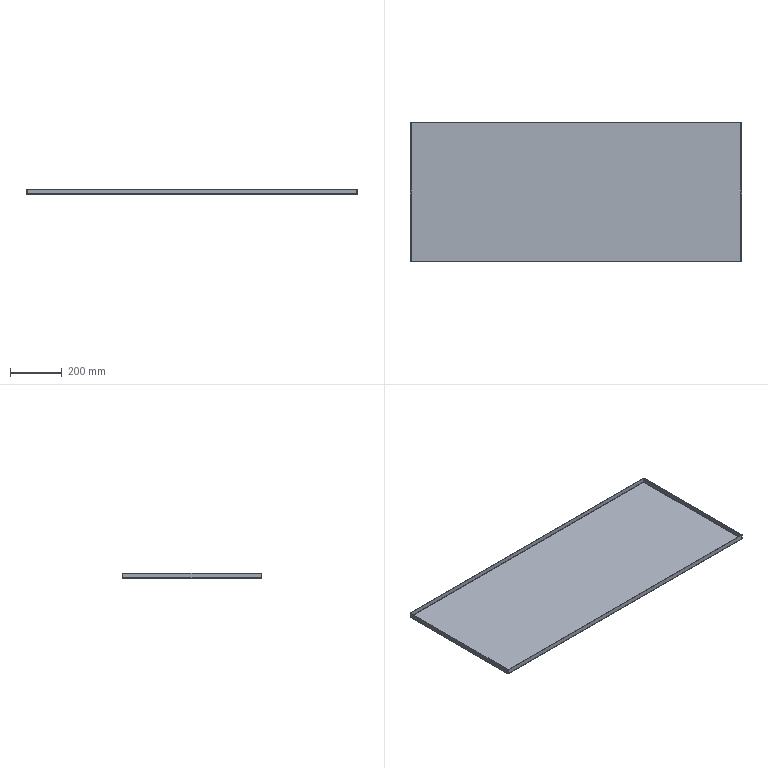Part | STEP file | Part 9 | 1 solid | 38 faces | box 1280 x 540 x 20 mm | volume 1507947 mm3 | plane 22 | spline 8 | cylinder 8 | commonest cylinder face diameters 1 x4 5 x4
STEP:
#1=CARTESIAN_POINT('',(-637.5,-267.5,-2.));
#2=VERTEX_POINT('',#1);
#3=CARTESIAN_POINT('',(-637.5,267.5,-2.));
#4=VERTEX_POINT('',#3);
#5=CARTESIAN_POINT('',(-637.5,-267.5,-2.));
#6=DIRECTION('',(0.,1.,0.));
#7=VECTOR('',#6,1000.);
#8=LINE('',#5,#7);
#9=EDGE_CURVE('',#2,#4,#8,.T.);
#10=ORIENTED_EDGE('',*,*,#9,.T.);
#11=CARTESIAN_POINT('',(637.5,267.5,-2.));
#12=VERTEX_POINT('',#11);
#13=CARTESIAN_POINT('',(-637.5,267.5,-2.));
#14=DIRECTION('',(1.,0.,0.));
#15=VECTOR('',#14,1000.);
#16=LINE('',#13,#15);
#17=EDGE_CURVE('',#4,#12,#16,.T.);
#18=ORIENTED_EDGE('',*,*,#17,.T.);
#19=CARTESIAN_POINT('',(637.5,-267.5,-2.));
#20=VERTEX_POINT('',#19);
#21=CARTESIAN_POINT('',(637.5,267.5,-2.));
#22=DIRECTION('',(0.,-1.,0.));
#23=VECTOR('',#22,1000.);
#24=LINE('',#21,#23);
#25=EDGE_CURVE('',#12,#20,#24,.T.);
#26=ORIENTED_EDGE('',*,*,#25,.T.);
#27=CARTESIAN_POINT('',(637.5,-267.5,-2.));
#28=DIRECTION('',(-1.,0.,0.));
#29=VECTOR('',#28,1000.);
#30=LINE('',#27,#29);
#31=EDGE_CURVE('',#20,#2,#30,.T.);
#32=ORIENTED_EDGE('',*,*,#31,.T.);
#33=EDGE_LOOP('',(#10,#18,#26,#32));
#34=FACE_OUTER_BOUND('',#33,.T.);
#35=CARTESIAN_POINT('',(0.,0.,-2.));
#36=DIRECTION('',(0.,0.,1.));
#37=DIRECTION('',(1.,0.,0.));
#38=AXIS2_PLACEMENT_3D('',#35,#36,#37);
#39=PLANE('',#38);
#40=ADVANCED_FACE('',(#34),#39,.F.);
#41=CARTESIAN_POINT('',(-637.5,267.5,0.));
#42=VERTEX_POINT('',#41);
#43=CARTESIAN_POINT('',(637.5,267.5,0.));
#44=VERTEX_POINT('',#43);
#45=CARTESIAN_POINT('',(-637.5,267.5,0.));
#46=DIRECTION('',(1.,0.,0.));
#47=VECTOR('',#46,1000.);
#48=LINE('',#45,#47);
#49=EDGE_CURVE('',#42,#44,#48,.T.);
#50=ORIENTED_EDGE('',*,*,#49,.F.);
#51=CARTESIAN_POINT('',(-637.5,-267.5,0.));
#52=VERTEX_POINT('',#51);
#53=CARTESIAN_POINT('',(-637.5,-267.5,0.));
#54=DIRECTION('',(0.,1.,0.));
#55=VECTOR('',#54,1000.);
#56=LINE('',#53,#55);
#57=EDGE_CURVE('',#52,#42,#56,.T.);
#58=ORIENTED_EDGE('',*,*,#57,.F.);
#59=CARTESIAN_POINT('',(637.5,-267.5,0.));
#60=VERTEX_POINT('',#59);
#61=CARTESIAN_POINT('',(637.5,-267.5,0.));
#62=DIRECTION('',(-1.,0.,0.));
#63=VECTOR('',#62,1000.);
#64=LINE('',#61,#63);
#65=EDGE_CURVE('',#60,#52,#64,.T.);
#66=ORIENTED_EDGE('',*,*,#65,.F.);
#67=CARTESIAN_POINT('',(637.5,267.5,0.));
#68=DIRECTION('',(0.,-1.,0.));
#69=VECTOR('',#68,1000.);
#70=LINE('',#67,#69);
#71=EDGE_CURVE('',#44,#60,#70,.T.);
#72=ORIENTED_EDGE('',*,*,#71,.F.);
#73=EDGE_LOOP('',(#50,#58,#66,#72));
#74=FACE_OUTER_BOUND('',#73,.T.);
#75=CARTESIAN_POINT('',(0.,0.,0.));
#76=DIRECTION('',(0.,0.,1.));
#77=DIRECTION('',(1.,0.,0.));
#78=AXIS2_PLACEMENT_3D('',#75,#76,#77);
#79=PLANE('',#78);
#80=ADVANCED_FACE('',(#74),#79,.T.);
#81=CARTESIAN_POINT('',(637.293,270.,0.5));
#82=VERTEX_POINT('',#81);
#83=CARTESIAN_POINT('',(637.293,268.,0.5));
#84=VERTEX_POINT('',#83);
#85=CARTESIAN_POINT('',(637.293,268.,0.5));
#86=DIRECTION('',(0.,-1.,0.));
#87=VECTOR('',#86,1000.);
#88=LINE('',#85,#87);
#89=EDGE_CURVE('',#82,#84,#88,.T.);
#90=ORIENTED_EDGE('',*,*,#89,.T.);
#91=CARTESIAN_POINT('',(637.5,267.5,0.));
#92=CARTESIAN_POINT('',(637.465,267.631,0.));
#93=CARTESIAN_POINT('',(637.431,267.761,0.05389));
#94=CARTESIAN_POINT('',(637.362,267.946,0.239));
#95=CARTESIAN_POINT('',(637.327,268.,0.3691));
#96=CARTESIAN_POINT('',(637.293,268.,0.5));
#97=B_SPLINE_CURVE_WITH_KNOTS('',3,(#91,#92,#93,#94,#95,#96),.UNSPECIFIED.,.F.,.F.,(4,2,4),(0.,0.5,1.),.UNSPECIFIED.);
#98=EDGE_CURVE('',#44,#84,#97,.T.);
#99=ORIENTED_EDGE('',*,*,#98,.F.);
#100=CARTESIAN_POINT('',(637.5,267.5,0.));
#101=DIRECTION('',(0.,0.,-1.));
#102=VECTOR('',#101,1000.);
#103=LINE('',#100,#102);
#104=EDGE_CURVE('',#44,#12,#103,.T.);
#105=ORIENTED_EDGE('',*,*,#104,.T.);
#106=CARTESIAN_POINT('',(637.5,267.5,-2.));
#107=CARTESIAN_POINT('',(637.483,267.827,-2.));
#108=CARTESIAN_POINT('',(637.465,268.154,-1.935));
#109=CARTESIAN_POINT('',(637.431,268.759,-1.684));
#110=CARTESIAN_POINT('',(637.414,269.036,-1.499));
#111=CARTESIAN_POINT('',(637.379,269.499,-1.036));
#112=CARTESIAN_POINT('',(637.362,269.684,-0.759));
#113=CARTESIAN_POINT('',(637.327,269.935,-0.1544));
#114=CARTESIAN_POINT('',(637.31,270.,0.1728));
#115=CARTESIAN_POINT('',(637.293,270.,0.5));
#116=B_SPLINE_CURVE_WITH_KNOTS('',3,(#106,#107,#108,#109,#110,#111,#112,#113,#114,#115),.UNSPECIFIED.,.F.,.F.,(4,2,2,2,4),(0.,0.25,0.5,0.75,1.),.UNSPECIFIED.);
#117=EDGE_CURVE('',#12,#82,#116,.T.);
#118=ORIENTED_EDGE('',*,*,#117,.T.);
#119=EDGE_LOOP('',(#90,#99,#105,#118));
#120=FACE_OUTER_BOUND('',#119,.T.);
#121=CARTESIAN_POINT('',(637.5,267.5,-2.02));
#122=CARTESIAN_POINT('',(637.483,267.83,-2.02));
#123=CARTESIAN_POINT('',(637.465,268.16,-1.954));
#124=CARTESIAN_POINT('',(637.431,268.769,-1.702));
#125=CARTESIAN_POINT('',(637.414,269.049,-1.515));
#126=CARTESIAN_POINT('',(637.379,269.515,-1.049));
#127=CARTESIAN_POINT('',(637.362,269.702,-0.7691));
#128=CARTESIAN_POINT('',(637.327,269.954,-0.1596));
#129=CARTESIAN_POINT('',(637.31,270.02,0.1701));
#130=CARTESIAN_POINT('',(637.293,270.02,0.5));
#131=CARTESIAN_POINT('',(637.5,267.5,-2.));
#132=CARTESIAN_POINT('',(637.483,267.827,-2.));
#133=CARTESIAN_POINT('',(637.465,268.154,-1.935));
#134=CARTESIAN_POINT('',(637.431,268.759,-1.684));
#135=CARTESIAN_POINT('',(637.414,269.036,-1.499));
#136=CARTESIAN_POINT('',(637.379,269.499,-1.036));
#137=CARTESIAN_POINT('',(637.362,269.684,-0.759));
#138=CARTESIAN_POINT('',(637.327,269.935,-0.1544));
#139=CARTESIAN_POINT('',(637.31,270.,0.1727));
#140=CARTESIAN_POINT('',(637.293,270.,0.5));
#141=CARTESIAN_POINT('',(637.5,267.5,0.));
#142=CARTESIAN_POINT('',(637.483,267.565,0.));
#143=CARTESIAN_POINT('',(637.465,267.631,0.01301));
#144=CARTESIAN_POINT('',(637.431,267.752,0.06311));
#145=CARTESIAN_POINT('',(637.414,267.807,0.1002));
#146=CARTESIAN_POINT('',(637.379,267.9,0.1927));
#147=CARTESIAN_POINT('',(637.362,267.937,0.2482));
#148=CARTESIAN_POINT('',(637.327,267.987,0.3691));
#149=CARTESIAN_POINT('',(637.31,268.,0.4345));
#150=CARTESIAN_POINT('',(637.293,268.,0.5));
#151=CARTESIAN_POINT('',(637.5,267.5,0.0202));
#152=CARTESIAN_POINT('',(637.483,267.563,0.0202));
#153=CARTESIAN_POINT('',(637.465,267.626,0.03269));
#154=CARTESIAN_POINT('',(637.431,267.742,0.08076));
#155=CARTESIAN_POINT('',(637.414,267.795,0.1163));
#156=CARTESIAN_POINT('',(637.379,267.884,0.2051));
#157=CARTESIAN_POINT('',(637.362,267.919,0.2584));
#158=CARTESIAN_POINT('',(637.327,267.967,0.3744));
#159=CARTESIAN_POINT('',(637.31,267.98,0.4372));
#160=CARTESIAN_POINT('',(637.293,267.98,0.5));
#161=B_SPLINE_SURFACE_WITH_KNOTS('',1,3,((#121,#122,#123,#124,#125,#126,#127,#128,#129,#130),(#131,#132,#133,#134,#135,#136,#137,#138,#139,#140),(#141,#142,#143,#144,#145,#146,#147,#148,#149,#150),(#151,#152,#153,#154,#155,#156,#157,#158,#159,#160)),.UNSPECIFIED.,.F.,.F.,.F.,(2,1,1,2),(4,2,2,2,4),(-0.01,0.,1.,1.01),(0.,0.25,0.5,0.75,1.),.UNSPECIFIED.);
#162=ADVANCED_FACE('',(#120),#161,.F.);
#163=CARTESIAN_POINT('',(-637.293,268.,0.5));
#164=VERTEX_POINT('',#163);
#165=CARTESIAN_POINT('',(-637.293,268.,0.5));
#166=CARTESIAN_POINT('',(-637.327,268.,0.3691));
#167=CARTESIAN_POINT('',(-637.362,267.946,0.239));
#168=CARTESIAN_POINT('',(-637.431,267.761,0.05389));
#169=CARTESIAN_POINT('',(-637.465,267.631,0.));
#170=CARTESIAN_POINT('',(-637.5,267.5,0.));
#171=B_SPLINE_CURVE_WITH_KNOTS('',3,(#165,#166,#167,#168,#169,#170),.UNSPECIFIED.,.F.,.F.,(4,2,4),(0.,0.5,1.),.UNSPECIFIED.);
#172=EDGE_CURVE('',#164,#42,#171,.T.);
#173=ORIENTED_EDGE('',*,*,#172,.F.);
#174=CARTESIAN_POINT('',(-637.293,270.,0.5));
#175=VERTEX_POINT('',#174);
#176=CARTESIAN_POINT('',(-637.293,268.,0.5));
#177=DIRECTION('',(0.,-1.,0.));
#178=VECTOR('',#177,1000.);
#179=LINE('',#176,#178);
#180=EDGE_CURVE('',#175,#164,#179,.T.);
#181=ORIENTED_EDGE('',*,*,#180,.F.);
#182=CARTESIAN_POINT('',(-637.293,270.,0.5));
#183=CARTESIAN_POINT('',(-637.31,270.,0.1728));
#184=CARTESIAN_POINT('',(-637.327,269.935,-0.1544));
#185=CARTESIAN_POINT('',(-637.362,269.684,-0.759));
#186=CARTESIAN_POINT('',(-637.379,269.499,-1.036));
#187=CARTESIAN_POINT('',(-637.414,269.036,-1.499));
#188=CARTESIAN_POINT('',(-637.431,268.759,-1.684));
#189=CARTESIAN_POINT('',(-637.465,268.154,-1.935));
#190=CARTESIAN_POINT('',(-637.483,267.827,-2.));
#191=CARTESIAN_POINT('',(-637.5,267.5,-2.));
#192=B_SPLINE_CURVE_WITH_KNOTS('',3,(#182,#183,#184,#185,#186,#187,#188,#189,#190,#191),.UNSPECIFIED.,.F.,.F.,(4,2,2,2,4),(0.,0.25,0.5,0.75,1.),.UNSPECIFIED.);
#193=EDGE_CURVE('',#175,#4,#192,.T.);
#194=ORIENTED_EDGE('',*,*,#193,.T.);
#195=CARTESIAN_POINT('',(-637.5,267.5,0.));
#196=DIRECTION('',(0.,0.,-1.));
#197=VECTOR('',#196,1000.);
#198=LINE('',#195,#197);
#199=EDGE_CURVE('',#42,#4,#198,.T.);
#200=ORIENTED_EDGE('',*,*,#199,.F.);
#201=EDGE_LOOP('',(#173,#181,#194,#200));
#202=FACE_OUTER_BOUND('',#201,.T.);
#203=CARTESIAN_POINT('',(-637.293,270.02,0.5));
#204=CARTESIAN_POINT('',(-637.31,270.02,0.1701));
#205=CARTESIAN_POINT('',(-637.327,269.954,-0.1596));
#206=CARTESIAN_POINT('',(-637.362,269.702,-0.7691));
#207=CARTESIAN_POINT('',(-637.379,269.515,-1.049));
#208=CARTESIAN_POINT('',(-637.414,269.049,-1.515));
#209=CARTESIAN_POINT('',(-637.431,268.769,-1.702));
#210=CARTESIAN_POINT('',(-637.465,268.16,-1.954));
#211=CARTESIAN_POINT('',(-637.483,267.83,-2.02));
#212=CARTESIAN_POINT('',(-637.5,267.5,-2.02));
#213=CARTESIAN_POINT('',(-637.293,270.,0.5));
#214=CARTESIAN_POINT('',(-637.31,270.,0.1727));
#215=CARTESIAN_POINT('',(-637.327,269.935,-0.1544));
#216=CARTESIAN_POINT('',(-637.362,269.684,-0.759));
#217=CARTESIAN_POINT('',(-637.379,269.499,-1.036));
#218=CARTESIAN_POINT('',(-637.414,269.036,-1.499));
#219=CARTESIAN_POINT('',(-637.431,268.759,-1.684));
#220=CARTESIAN_POINT('',(-637.465,268.154,-1.935));
#221=CARTESIAN_POINT('',(-637.483,267.827,-2.));
#222=CARTESIAN_POINT('',(-637.5,267.5,-2.));
#223=CARTESIAN_POINT('',(-637.293,268.,0.5));
#224=CARTESIAN_POINT('',(-637.31,268.,0.4345));
#225=CARTESIAN_POINT('',(-637.327,267.987,0.3691));
#226=CARTESIAN_POINT('',(-637.362,267.937,0.2482));
#227=CARTESIAN_POINT('',(-637.379,267.9,0.1927));
#228=CARTESIAN_POINT('',(-637.414,267.807,0.1002));
#229=CARTESIAN_POINT('',(-637.431,267.752,0.06311));
#230=CARTESIAN_POINT('',(-637.465,267.631,0.01301));
#231=CARTESIAN_POINT('',(-637.483,267.565,0.));
#232=CARTESIAN_POINT('',(-637.5,267.5,0.));
#233=CARTESIAN_POINT('',(-637.293,267.98,0.5));
#234=CARTESIAN_POINT('',(-637.31,267.98,0.4372));
#235=CARTESIAN_POINT('',(-637.327,267.967,0.3744));
#236=CARTESIAN_POINT('',(-637.362,267.919,0.2584));
#237=CARTESIAN_POINT('',(-637.379,267.884,0.2051));
#238=CARTESIAN_POINT('',(-637.414,267.795,0.1163));
#239=CARTESIAN_POINT('',(-637.431,267.742,0.08076));
#240=CARTESIAN_POINT('',(-637.465,267.626,0.03269));
#241=CARTESIAN_POINT('',(-637.483,267.563,0.0202));
#242=CARTESIAN_POINT('',(-637.5,267.5,0.0202));
#243=B_SPLINE_SURFACE_WITH_KNOTS('',1,3,((#203,#204,#205,#206,#207,#208,#209,#210,#211,#212),(#213,#214,#215,#216,#217,#218,#219,#220,#221,#222),(#223,#224,#225,#226,#227,#228,#229,#230,#231,#232),(#233,#234,#235,#236,#237,#238,#239,#240,#241,#242)),.UNSPECIFIED.,.F.,.F.,.F.,(2,1,1,2),(4,2,2,2,4),(-0.01,0.,1.,1.01),(0.,0.25,0.5,0.75,1.),.UNSPECIFIED.);
#244=ADVANCED_FACE('',(#202),#243,.F.);
#245=ORIENTED_EDGE('',*,*,#17,.F.);
#246=ORIENTED_EDGE('',*,*,#193,.F.);
#247=CARTESIAN_POINT('',(0.,270.,0.5));
#248=DIRECTION('',(-1.,0.,0.));
#249=VECTOR('',#248,1000.);
#250=LINE('',#247,#249);
#251=EDGE_CURVE('',#82,#175,#250,.T.);
#252=ORIENTED_EDGE('',*,*,#251,.F.);
#253=ORIENTED_EDGE('',*,*,#117,.F.);
#254=EDGE_LOOP('',(#245,#246,#252,#253));
#255=FACE_OUTER_BOUND('',#254,.T.);
#256=CARTESIAN_POINT('',(-637.5,267.5,0.5));
#257=DIRECTION('',(-1.,0.,0.));
#258=DIRECTION('',(0.,1.,0.));
#259=AXIS2_PLACEMENT_3D('',#256,#257,#258);
#260=CYLINDRICAL_SURFACE('',#259,2.5);
#261=ADVANCED_FACE('',(#255),#260,.T.);
#262=ORIENTED_EDGE('',*,*,#49,.T.);
#263=ORIENTED_EDGE('',*,*,#98,.T.);
#264=CARTESIAN_POINT('',(640.,268.,0.5));
#265=DIRECTION('',(-1.,0.,0.));
#266=VECTOR('',#265,1000.);
#267=LINE('',#264,#266);
#268=EDGE_CURVE('',#84,#164,#267,.T.);
#269=ORIENTED_EDGE('',*,*,#268,.T.);
#270=ORIENTED_EDGE('',*,*,#172,.T.);
#271=EDGE_LOOP('',(#262,#263,#269,#270));
#272=FACE_OUTER_BOUND('',#271,.T.);
#273=CARTESIAN_POINT('',(-637.5,267.5,0.5));
#274=DIRECTION('',(-1.,0.,0.));
#275=DIRECTION('',(0.,1.,0.));
#276=AXIS2_PLACEMENT_3D('',#273,#274,#275);
#277=CYLINDRICAL_SURFACE('',#276,0.5);
#278=ADVANCED_FACE('',(#272),#277,.F.);
#279=CARTESIAN_POINT('',(637.293,268.,18.));
#280=VERTEX_POINT('',#279);
#281=CARTESIAN_POINT('',(637.293,270.,18.));
#282=VERTEX_POINT('',#281);
#283=CARTESIAN_POINT('',(637.293,270.,18.));
#284=DIRECTION('',(0.,1.,0.));
#285=VECTOR('',#284,1000.);
#286=LINE('',#283,#285);
#287=EDGE_CURVE('',#280,#282,#286,.T.);
#288=ORIENTED_EDGE('',*,*,#287,.F.);
#289=CARTESIAN_POINT('',(637.293,268.,0.));
#290=DIRECTION('',(0.,0.,1.));
#291=VECTOR('',#290,1000.);
#292=LINE('',#289,#291);
#293=EDGE_CURVE('',#84,#280,#292,.T.);
#294=ORIENTED_EDGE('',*,*,#293,.F.);
#295=ORIENTED_EDGE('',*,*,#89,.F.);
#296=CARTESIAN_POINT('',(637.293,270.,0.));
#297=DIRECTION('',(0.,0.,-1.));
#298=VECTOR('',#297,1000.);
#299=LINE('',#296,#298);
#300=EDGE_CURVE('',#282,#82,#299,.T.);
#301=ORIENTED_EDGE('',*,*,#300,.F.);
#302=EDGE_LOOP('',(#288,#294,#295,#301));
#303=FACE_OUTER_BOUND('',#302,.T.);
#304=CARTESIAN_POINT('',(637.293,268.,0.));
#305=DIRECTION('',(1.,0.,0.));
#306=DIRECTION('',(0.,0.,-1.));
#307=AXIS2_PLACEMENT_3D('',#304,#305,#306);
#308=PLANE('',#307);
#309=ADVANCED_FACE('',(#303),#308,.T.);
#310=CARTESIAN_POINT('',(-637.293,270.,18.));
#311=VERTEX_POINT('',#310);
#312=CARTESIAN_POINT('',(-637.293,270.,0.));
#313=DIRECTION('',(0.,0.,-1.));
#314=VECTOR('',#313,1000.);
#315=LINE('',#312,#314);
#316=EDGE_CURVE('',#311,#175,#315,.T.);
#317=ORIENTED_EDGE('',*,*,#316,.F.);
#318=CARTESIAN_POINT('',(-640.,270.,18.));
#319=DIRECTION('',(-1.,0.,0.));
#320=VECTOR('',#319,1000.);
#321=LINE('',#318,#320);
#322=EDGE_CURVE('',#282,#311,#321,.T.);
#323=ORIENTED_EDGE('',*,*,#322,.F.);
#324=ORIENTED_EDGE('',*,*,#300,.T.);
#325=ORIENTED_EDGE('',*,*,#251,.T.);
#326=EDGE_LOOP('',(#317,#323,#324,#325));
#327=FACE_OUTER_BOUND('',#326,.T.);
#328=CARTESIAN_POINT('',(0.,270.,0.));
#329=DIRECTION('',(0.,1.,0.));
#330=DIRECTION('',(0.,0.,1.));
#331=AXIS2_PLACEMENT_3D('',#328,#329,#330);
#332=PLANE('',#331);
#333=ADVANCED_FACE('',(#327),#332,.T.);
#334=CARTESIAN_POINT('',(-637.293,268.,18.));
#335=VERTEX_POINT('',#334);
#336=CARTESIAN_POINT('',(0.,268.,18.));
#337=DIRECTION('',(-1.,0.,0.));
#338=VECTOR('',#337,1000.);
#339=LINE('',#336,#338);
#340=EDGE_CURVE('',#280,#335,#339,.T.);
#341=ORIENTED_EDGE('',*,*,#340,.T.);
#342=CARTESIAN_POINT('',(-637.293,268.,0.));
#343=DIRECTION('',(0.,0.,1.));
#344=VECTOR('',#343,1000.);
#345=LINE('',#342,#344);
#346=EDGE_CURVE('',#164,#335,#345,.T.);
#347=ORIENTED_EDGE('',*,*,#346,.F.);
#348=ORIENTED_EDGE('',*,*,#268,.F.);
#349=ORIENTED_EDGE('',*,*,#293,.T.);
#350=EDGE_LOOP('',(#341,#347,#348,#349));
#351=FACE_OUTER_BOUND('',#350,.T.);
#352=CARTESIAN_POINT('',(0.,268.,0.));
#353=DIRECTION('',(0.,1.,0.));
#354=DIRECTION('',(0.,0.,1.));
#355=AXIS2_PLACEMENT_3D('',#352,#353,#354);
#356=PLANE('',#355);
#357=ADVANCED_FACE('',(#351),#356,.F.);
#358=CARTESIAN_POINT('',(-637.293,268.,18.));
#359=DIRECTION('',(0.,1.,0.));
#360=VECTOR('',#359,1000.);
#361=LINE('',#358,#360);
#362=EDGE_CURVE('',#335,#311,#361,.T.);
#363=ORIENTED_EDGE('',*,*,#362,.F.);
#364=ORIENTED_EDGE('',*,*,#340,.F.);
#365=ORIENTED_EDGE('',*,*,#287,.T.);
#366=ORIENTED_EDGE('',*,*,#322,.T.);
#367=EDGE_LOOP('',(#363,#364,#365,#366));
#368=FACE_OUTER_BOUND('',#367,.T.);
#369=CARTESIAN_POINT('',(-640.,270.,18.));
#370=DIRECTION('',(0.,0.,1.));
#371=DIRECTION('',(0.,-1.,0.));
#372=AXIS2_PLACEMENT_3D('',#369,#370,#371);
#373=PLANE('',#372);
#374=ADVANCED_FACE('',(#368),#373,.T.);
#375=ORIENTED_EDGE('',*,*,#346,.T.);
#376=ORIENTED_EDGE('',*,*,#362,.T.);
#377=ORIENTED_EDGE('',*,*,#316,.T.);
#378=ORIENTED_EDGE('',*,*,#180,.T.);
#379=EDGE_LOOP('',(#375,#376,#377,#378));
#380=FACE_OUTER_BOUND('',#379,.T.);
#381=CARTESIAN_POINT('',(-637.293,268.,0.));
#382=DIRECTION('',(1.,0.,0.));
#383=DIRECTION('',(0.,0.,-1.));
#384=AXIS2_PLACEMENT_3D('',#381,#382,#383);
#385=PLANE('',#384);
#386=ADVANCED_FACE('',(#380),#385,.F.);
#387=CARTESIAN_POINT('',(640.,-267.293,0.5));
#388=VERTEX_POINT('',#387);
#389=CARTESIAN_POINT('',(638.,-267.293,0.5));
#390=VERTEX_POINT('',#389);
#391=CARTESIAN_POINT('',(638.,-267.293,0.5));
#392=DIRECTION('',(-1.,0.,0.));
#393=VECTOR('',#392,1000.);
#394=LINE('',#391,#393);
#395=EDGE_CURVE('',#388,#390,#394,.T.);
#396=ORIENTED_EDGE('',*,*,#395,.T.);
#397=CARTESIAN_POINT('',(637.5,-267.5,0.));
#398=CARTESIAN_POINT('',(637.631,-267.465,0.));
#399=CARTESIAN_POINT('',(637.761,-267.431,0.05389));
#400=CARTESIAN_POINT('',(637.946,-267.362,0.239));
#401=CARTESIAN_POINT('',(638.,-267.327,0.3691));
#402=CARTESIAN_POINT('',(638.,-267.293,0.5));
#403=B_SPLINE_CURVE_WITH_KNOTS('',3,(#397,#398,#399,#400,#401,#402),.UNSPECIFIED.,.F.,.F.,(4,2,4),(0.,0.5,1.),.UNSPECIFIED.);
#404=EDGE_CURVE('',#60,#390,#403,.T.);
#405=ORIENTED_EDGE('',*,*,#404,.F.);
#406=CARTESIAN_POINT('',(637.5,-267.5,0.));
#407=DIRECTION('',(0.,0.,-1.));
#408=VECTOR('',#407,1000.);
#409=LINE('',#406,#408);
#410=EDGE_CURVE('',#60,#20,#409,.T.);
#411=ORIENTED_EDGE('',*,*,#410,.T.);
#412=CARTESIAN_POINT('',(637.5,-267.5,-2.));
#413=CARTESIAN_POINT('',(637.827,-267.483,-2.));
#414=CARTESIAN_POINT('',(638.154,-267.465,-1.935));
#415=CARTESIAN_POINT('',(638.759,-267.431,-1.684));
#416=CARTESIAN_POINT('',(639.036,-267.414,-1.499));
#417=CARTESIAN_POINT('',(639.499,-267.379,-1.036));
#418=CARTESIAN_POINT('',(639.684,-267.362,-0.759));
#419=CARTESIAN_POINT('',(639.935,-267.327,-0.1544));
#420=CARTESIAN_POINT('',(640.,-267.31,0.1728));
#421=CARTESIAN_POINT('',(640.,-267.293,0.5));
#422=B_SPLINE_CURVE_WITH_KNOTS('',3,(#412,#413,#414,#415,#416,#417,#418,#419,#420,#421),.UNSPECIFIED.,.F.,.F.,(4,2,2,2,4),(0.,0.25,0.5,0.75,1.),.UNSPECIFIED.);
#423=EDGE_CURVE('',#20,#388,#422,.T.);
#424=ORIENTED_EDGE('',*,*,#423,.T.);
#425=EDGE_LOOP('',(#396,#405,#411,#424));
#426=FACE_OUTER_BOUND('',#425,.T.);
#427=CARTESIAN_POINT('',(637.5,-267.5,-2.02));
#428=CARTESIAN_POINT('',(637.83,-267.483,-2.02));
#429=CARTESIAN_POINT('',(638.16,-267.465,-1.954));
#430=CARTESIAN_POINT('',(638.769,-267.431,-1.702));
#431=CARTESIAN_POINT('',(639.049,-267.414,-1.515));
#432=CARTESIAN_POINT('',(639.515,-267.379,-1.049));
#433=CARTESIAN_POINT('',(639.702,-267.362,-0.7691));
#434=CARTESIAN_POINT('',(639.954,-267.327,-0.1596));
#435=CARTESIAN_POINT('',(640.02,-267.31,0.1701));
#436=CARTESIAN_POINT('',(640.02,-267.293,0.5));
#437=CARTESIAN_POINT('',(637.5,-267.5,-2.));
#438=CARTESIAN_POINT('',(637.827,-267.483,-2.));
#439=CARTESIAN_POINT('',(638.154,-267.465,-1.935));
#440=CARTESIAN_POINT('',(638.759,-267.431,-1.684));
#441=CARTESIAN_POINT('',(639.036,-267.414,-1.499));
#442=CARTESIAN_POINT('',(639.499,-267.379,-1.036));
#443=CARTESIAN_POINT('',(639.684,-267.362,-0.759));
#444=CARTESIAN_POINT('',(639.935,-267.327,-0.1544));
#445=CARTESIAN_POINT('',(640.,-267.31,0.1727));
#446=CARTESIAN_POINT('',(640.,-267.293,0.5));
#447=CARTESIAN_POINT('',(637.5,-267.5,0.));
#448=CARTESIAN_POINT('',(637.565,-267.483,0.));
#449=CARTESIAN_POINT('',(637.631,-267.465,0.01301));
#450=CARTESIAN_POINT('',(637.752,-267.431,0.06311));
#451=CARTESIAN_POINT('',(637.807,-267.414,0.1002));
#452=CARTESIAN_POINT('',(637.9,-267.379,0.1927));
#453=CARTESIAN_POINT('',(637.937,-267.362,0.2482));
#454=CARTESIAN_POINT('',(637.987,-267.327,0.3691));
#455=CARTESIAN_POINT('',(638.,-267.31,0.4345));
#456=CARTESIAN_POINT('',(638.,-267.293,0.5));
#457=CARTESIAN_POINT('',(637.5,-267.5,0.0202));
#458=CARTESIAN_POINT('',(637.563,-267.483,0.0202));
#459=CARTESIAN_POINT('',(637.626,-267.465,0.03269));
#460=CARTESIAN_POINT('',(637.742,-267.431,0.08076));
#461=CARTESIAN_POINT('',(637.795,-267.414,0.1163));
#462=CARTESIAN_POINT('',(637.884,-267.379,0.2051));
#463=CARTESIAN_POINT('',(637.919,-267.362,0.2584));
#464=CARTESIAN_POINT('',(637.967,-267.327,0.3744));
#465=CARTESIAN_POINT('',(637.98,-267.31,0.4372));
#466=CARTESIAN_POINT('',(637.98,-267.293,0.5));
#467=B_SPLINE_SURFACE_WITH_KNOTS('',1,3,((#427,#428,#429,#430,#431,#432,#433,#434,#435,#436),(#437,#438,#439,#440,#441,#442,#443,#444,#445,#446),(#447,#448,#449,#450,#451,#452,#453,#454,#455,#456),(#457,#458,#459,#460,#461,#462,#463,#464,#465,#466)),.UNSPECIFIED.,.F.,.F.,.F.,(2,1,1,2),(4,2,2,2,4),(-0.01,0.,1.,1.01),(0.,0.25,0.5,0.75,1.),.UNSPECIFIED.);
#468=ADVANCED_FACE('',(#426),#467,.F.);
#469=CARTESIAN_POINT('',(638.,267.293,0.5));
#470=VERTEX_POINT('',#469);
#471=CARTESIAN_POINT('',(638.,267.293,0.5));
#472=CARTESIAN_POINT('',(638.,267.327,0.3691));
#473=CARTESIAN_POINT('',(637.946,267.362,0.239));
#474=CARTESIAN_POINT('',(637.761,267.431,0.05389));
#475=CARTESIAN_POINT('',(637.631,267.465,0.));
#476=CARTESIAN_POINT('',(637.5,267.5,0.));
#477=B_SPLINE_CURVE_WITH_KNOTS('',3,(#471,#472,#473,#474,#475,#476),.UNSPECIFIED.,.F.,.F.,(4,2,4),(0.,0.5,1.),.UNSPECIFIED.);
#478=EDGE_CURVE('',#470,#44,#477,.T.);
#479=ORIENTED_EDGE('',*,*,#478,.F.);
#480=CARTESIAN_POINT('',(640.,267.293,0.5));
#481=VERTEX_POINT('',#480);
#482=CARTESIAN_POINT('',(638.,267.293,0.5));
#483=DIRECTION('',(-1.,0.,0.));
#484=VECTOR('',#483,1000.);
#485=LINE('',#482,#484);
#486=EDGE_CURVE('',#481,#470,#485,.T.);
#487=ORIENTED_EDGE('',*,*,#486,.F.);
#488=CARTESIAN_POINT('',(640.,267.293,0.5));
#489=CARTESIAN_POINT('',(640.,267.31,0.1728));
#490=CARTESIAN_POINT('',(639.935,267.327,-0.1544));
#491=CARTESIAN_POINT('',(639.684,267.362,-0.759));
#492=CARTESIAN_POINT('',(639.499,267.379,-1.036));
#493=CARTESIAN_POINT('',(639.036,267.414,-1.499));
#494=CARTESIAN_POINT('',(638.759,267.431,-1.684));
#495=CARTESIAN_POINT('',(638.154,267.465,-1.935));
#496=CARTESIAN_POINT('',(637.827,267.483,-2.));
#497=CARTESIAN_POINT('',(637.5,267.5,-2.));
#498=B_SPLINE_CURVE_WITH_KNOTS('',3,(#488,#489,#490,#491,#492,#493,#494,#495,#496,#497),.UNSPECIFIED.,.F.,.F.,(4,2,2,2,4),(0.,0.25,0.5,0.75,1.),.UNSPECIFIED.);
#499=EDGE_CURVE('',#481,#12,#498,.T.);
#500=ORIENTED_EDGE('',*,*,#499,.T.);
#501=ORIENTED_EDGE('',*,*,#104,.F.);
#502=EDGE_LOOP('',(#479,#487,#500,#501));
#503=FACE_OUTER_BOUND('',#502,.T.);
#504=CARTESIAN_POINT('',(640.02,267.293,0.5));
#505=CARTESIAN_POINT('',(640.02,267.31,0.1701));
#506=CARTESIAN_POINT('',(639.954,267.327,-0.1596));
#507=CARTESIAN_POINT('',(639.702,267.362,-0.7691));
#508=CARTESIAN_POINT('',(639.515,267.379,-1.049));
#509=CARTESIAN_POINT('',(639.049,267.414,-1.515));
#510=CARTESIAN_POINT('',(638.769,267.431,-1.702));
#511=CARTESIAN_POINT('',(638.16,267.465,-1.954));
#512=CARTESIAN_POINT('',(637.83,267.483,-2.02));
#513=CARTESIAN_POINT('',(637.5,267.5,-2.02));
#514=CARTESIAN_POINT('',(640.,267.293,0.5));
#515=CARTESIAN_POINT('',(640.,267.31,0.1727));
#516=CARTESIAN_POINT('',(639.935,267.327,-0.1544));
#517=CARTESIAN_POINT('',(639.684,267.362,-0.759));
#518=CARTESIAN_POINT('',(639.499,267.379,-1.036));
#519=CARTESIAN_POINT('',(639.036,267.414,-1.499));
#520=CARTESIAN_POINT('',(638.759,267.431,-1.684));
#521=CARTESIAN_POINT('',(638.154,267.465,-1.935));
#522=CARTESIAN_POINT('',(637.827,267.483,-2.));
#523=CARTESIAN_POINT('',(637.5,267.5,-2.));
#524=CARTESIAN_POINT('',(638.,267.293,0.5));
#525=CARTESIAN_POINT('',(638.,267.31,0.4345));
#526=CARTESIAN_POINT('',(637.987,267.327,0.3691));
#527=CARTESIAN_POINT('',(637.937,267.362,0.2482));
#528=CARTESIAN_POINT('',(637.9,267.379,0.1927));
#529=CARTESIAN_POINT('',(637.807,267.414,0.1002));
#530=CARTESIAN_POINT('',(637.752,267.431,0.06311));
#531=CARTESIAN_POINT('',(637.631,267.465,0.01301));
#532=CARTESIAN_POINT('',(637.565,267.483,0.));
#533=CARTESIAN_POINT('',(637.5,267.5,0.));
#534=CARTESIAN_POINT('',(637.98,267.293,0.5));
#535=CARTESIAN_POINT('',(637.98,267.31,0.4372));
#536=CARTESIAN_POINT('',(637.967,267.327,0.3744));
#537=CARTESIAN_POINT('',(637.919,267.362,0.2584));
#538=CARTESIAN_POINT('',(637.884,267.379,0.2051));
#539=CARTESIAN_POINT('',(637.795,267.414,0.1163));
#540=CARTESIAN_POINT('',(637.742,267.431,0.08076));
#541=CARTESIAN_POINT('',(637.626,267.465,0.03269));
#542=CARTESIAN_POINT('',(637.563,267.483,0.0202));
#543=CARTESIAN_POINT('',(637.5,267.5,0.0202));
#544=B_SPLINE_SURFACE_WITH_KNOTS('',1,3,((#504,#505,#506,#507,#508,#509,#510,#511,#512,#513),(#514,#515,#516,#517,#518,#519,#520,#521,#522,#523),(#524,#525,#526,#527,#528,#529,#530,#531,#532,#533),(#534,#535,#536,#537,#538,#539,#540,#541,#542,#543)),.UNSPECIFIED.,.F.,.F.,.F.,(2,1,1,2),(4,2,2,2,4),(-0.01,0.,1.,1.01),(0.,0.25,0.5,0.75,1.),.UNSPECIFIED.);
#545=ADVANCED_FACE('',(#503),#544,.F.);
#546=ORIENTED_EDGE('',*,*,#25,.F.);
#547=ORIENTED_EDGE('',*,*,#499,.F.);
#548=CARTESIAN_POINT('',(640.,-270.,0.5));
#549=DIRECTION('',(0.,-1.,0.));
#550=VECTOR('',#549,1000.);
#551=LINE('',#548,#550);
#552=EDGE_CURVE('',#481,#388,#551,.T.);
#553=ORIENTED_EDGE('',*,*,#552,.T.);
#554=ORIENTED_EDGE('',*,*,#423,.F.);
#555=EDGE_LOOP('',(#546,#547,#553,#554));
#556=FACE_OUTER_BOUND('',#555,.T.);
#557=CARTESIAN_POINT('',(637.5,267.5,0.5));
#558=DIRECTION('',(0.,1.,0.));
#559=DIRECTION('',(1.,0.,0.));
#560=AXIS2_PLACEMENT_3D('',#557,#558,#559);
#561=CYLINDRICAL_SURFACE('',#560,2.5);
#562=ADVANCED_FACE('',(#556),#561,.T.);
#563=ORIENTED_EDGE('',*,*,#71,.T.);
#564=ORIENTED_EDGE('',*,*,#404,.T.);
#565=CARTESIAN_POINT('',(638.,-270.,0.5));
#566=DIRECTION('',(0.,1.,0.));
#567=VECTOR('',#566,1000.);
#568=LINE('',#565,#567);
#569=EDGE_CURVE('',#390,#470,#568,.T.);
#570=ORIENTED_EDGE('',*,*,#569,.T.);
#571=ORIENTED_EDGE('',*,*,#478,.T.);
#572=EDGE_LOOP('',(#563,#564,#570,#571));
#573=FACE_OUTER_BOUND('',#572,.T.);
#574=CARTESIAN_POINT('',(637.5,267.5,0.5));
#575=DIRECTION('',(0.,1.,0.));
#576=DIRECTION('',(1.,0.,0.));
#577=AXIS2_PLACEMENT_3D('',#574,#575,#576);
#578=CYLINDRICAL_SURFACE('',#577,0.5);
#579=ADVANCED_FACE('',(#573),#578,.F.);
#580=CARTESIAN_POINT('',(638.,-267.293,18.));
#581=VERTEX_POINT('',#580);
#582=CARTESIAN_POINT('',(640.,-267.293,18.));
#583=VERTEX_POINT('',#582);
#584=CARTESIAN_POINT('',(640.,-267.293,18.));
#585=DIRECTION('',(1.,0.,0.));
#586=VECTOR('',#585,1000.);
#587=LINE('',#584,#586);
#588=EDGE_CURVE('',#581,#583,#587,.T.);
#589=ORIENTED_EDGE('',*,*,#588,.F.);
#590=CARTESIAN_POINT('',(638.,-267.293,0.));
#591=DIRECTION('',(0.,0.,1.));
#592=VECTOR('',#591,1000.);
#593=LINE('',#590,#592);
#594=EDGE_CURVE('',#390,#581,#593,.T.);
#595=ORIENTED_EDGE('',*,*,#594,.F.);
#596=ORIENTED_EDGE('',*,*,#395,.F.);
#597=CARTESIAN_POINT('',(640.,-267.293,0.));
#598=DIRECTION('',(0.,0.,1.));
#599=VECTOR('',#598,1000.);
#600=LINE('',#597,#599);
#601=EDGE_CURVE('',#388,#583,#600,.T.);
#602=ORIENTED_EDGE('',*,*,#601,.T.);
#603=EDGE_LOOP('',(#589,#595,#596,#602));
#604=FACE_OUTER_BOUND('',#603,.T.);
#605=CARTESIAN_POINT('',(638.,-267.293,0.));
#606=DIRECTION('',(0.,-1.,0.));
#607=DIRECTION('',(0.,0.,-1.));
#608=AXIS2_PLACEMENT_3D('',#605,#606,#607);
#609=PLANE('',#608);
#610=ADVANCED_FACE('',(#604),#609,.T.);
#611=ORIENTED_EDGE('',*,*,#552,.F.);
#612=CARTESIAN_POINT('',(640.,267.293,18.));
#613=VERTEX_POINT('',#612);
#614=CARTESIAN_POINT('',(640.,267.293,0.));
#615=DIRECTION('',(0.,0.,1.));
#616=VECTOR('',#615,1000.);
#617=LINE('',#614,#616);
#618=EDGE_CURVE('',#481,#613,#617,.T.);
#619=ORIENTED_EDGE('',*,*,#618,.T.);
#620=CARTESIAN_POINT('',(640.,-270.,18.));
#621=DIRECTION('',(0.,1.,0.));
#622=VECTOR('',#621,1000.);
#623=LINE('',#620,#622);
#624=EDGE_CURVE('',#583,#613,#623,.T.);
#625=ORIENTED_EDGE('',*,*,#624,.F.);
#626=ORIENTED_EDGE('',*,*,#601,.F.);
#627=EDGE_LOOP('',(#611,#619,#625,#626));
#628=FACE_OUTER_BOUND('',#627,.T.);
#629=CARTESIAN_POINT('',(640.,0.,0.));
#630=DIRECTION('',(-1.,0.,0.));
#631=DIRECTION('',(0.,-1.,0.));
#632=AXIS2_PLACEMENT_3D('',#629,#630,#631);
#633=PLANE('',#632);
#634=ADVANCED_FACE('',(#628),#633,.F.);
#635=CARTESIAN_POINT('',(638.,267.293,18.));
#636=VERTEX_POINT('',#635);
#637=CARTESIAN_POINT('',(638.,267.293,0.));
#638=DIRECTION('',(0.,0.,1.));
#639=VECTOR('',#638,1000.);
#640=LINE('',#637,#639);
#641=EDGE_CURVE('',#470,#636,#640,.T.);
#642=ORIENTED_EDGE('',*,*,#641,.F.);
#643=ORIENTED_EDGE('',*,*,#569,.F.);
#644=ORIENTED_EDGE('',*,*,#594,.T.);
#645=CARTESIAN_POINT('',(638.,0.,18.));
#646=DIRECTION('',(0.,1.,0.));
#647=VECTOR('',#646,1000.);
#648=LINE('',#645,#647);
#649=EDGE_CURVE('',#581,#636,#648,.T.);
#650=ORIENTED_EDGE('',*,*,#649,.T.);
#651=EDGE_LOOP('',(#642,#643,#644,#650));
#652=FACE_OUTER_BOUND('',#651,.T.);
#653=CARTESIAN_POINT('',(638.,0.,0.));
#654=DIRECTION('',(-1.,0.,0.));
#655=DIRECTION('',(0.,-1.,0.));
#656=AXIS2_PLACEMENT_3D('',#653,#654,#655);
#657=PLANE('',#656);
#658=ADVANCED_FACE('',(#652),#657,.T.);
#659=CARTESIAN_POINT('',(638.,267.293,18.));
#660=DIRECTION('',(1.,0.,0.));
#661=VECTOR('',#660,1000.);
#662=LINE('',#659,#661);
#663=EDGE_CURVE('',#636,#613,#662,.T.);
#664=ORIENTED_EDGE('',*,*,#663,.F.);
#665=ORIENTED_EDGE('',*,*,#649,.F.);
#666=ORIENTED_EDGE('',*,*,#588,.T.);
#667=ORIENTED_EDGE('',*,*,#624,.T.);
#668=EDGE_LOOP('',(#664,#665,#666,#667));
#669=FACE_OUTER_BOUND('',#668,.T.);
#670=CARTESIAN_POINT('',(640.,-270.,18.));
#671=DIRECTION('',(0.,0.,1.));
#672=DIRECTION('',(1.,0.,0.));
#673=AXIS2_PLACEMENT_3D('',#670,#671,#672);
#674=PLANE('',#673);
#675=ADVANCED_FACE('',(#669),#674,.T.);
#676=ORIENTED_EDGE('',*,*,#641,.T.);
#677=ORIENTED_EDGE('',*,*,#663,.T.);
#678=ORIENTED_EDGE('',*,*,#618,.F.);
#679=ORIENTED_EDGE('',*,*,#486,.T.);
#680=EDGE_LOOP('',(#676,#677,#678,#679));
#681=FACE_OUTER_BOUND('',#680,.T.);
#682=CARTESIAN_POINT('',(638.,267.293,0.));
#683=DIRECTION('',(0.,-1.,0.));
#684=DIRECTION('',(0.,0.,-1.));
#685=AXIS2_PLACEMENT_3D('',#682,#683,#684);
#686=PLANE('',#685);
#687=ADVANCED_FACE('',(#681),#686,.F.);
#688=CARTESIAN_POINT('',(-637.293,-270.,0.5));
#689=VERTEX_POINT('',#688);
#690=CARTESIAN_POINT('',(-637.293,-268.,0.5));
#691=VERTEX_POINT('',#690);
#692=CARTESIAN_POINT('',(-637.293,-268.,0.5));
#693=DIRECTION('',(0.,1.,0.));
#694=VECTOR('',#693,1000.);
#695=LINE('',#692,#694);
#696=EDGE_CURVE('',#689,#691,#695,.T.);
#697=ORIENTED_EDGE('',*,*,#696,.T.);
#698=CARTESIAN_POINT('',(-637.5,-267.5,0.));
#699=CARTESIAN_POINT('',(-637.465,-267.631,0.));
#700=CARTESIAN_POINT('',(-637.431,-267.761,0.05389));
#701=CARTESIAN_POINT('',(-637.362,-267.946,0.239));
#702=CARTESIAN_POINT('',(-637.327,-268.,0.3691));
#703=CARTESIAN_POINT('',(-637.293,-268.,0.5));
#704=B_SPLINE_CURVE_WITH_KNOTS('',3,(#698,#699,#700,#701,#702,#703),.UNSPECIFIED.,.F.,.F.,(4,2,4),(0.,0.5,1.),.UNSPECIFIED.);
#705=EDGE_CURVE('',#52,#691,#704,.T.);
#706=ORIENTED_EDGE('',*,*,#705,.F.);
#707=CARTESIAN_POINT('',(-637.5,-267.5,0.));
#708=DIRECTION('',(0.,0.,-1.));
#709=VECTOR('',#708,1000.);
#710=LINE('',#707,#709);
#711=EDGE_CURVE('',#52,#2,#710,.T.);
#712=ORIENTED_EDGE('',*,*,#711,.T.);
#713=CARTESIAN_POINT('',(-637.5,-267.5,-2.));
#714=CARTESIAN_POINT('',(-637.483,-267.827,-2.));
#715=CARTESIAN_POINT('',(-637.465,-268.154,-1.935));
#716=CARTESIAN_POINT('',(-637.431,-268.759,-1.684));
#717=CARTESIAN_POINT('',(-637.414,-269.036,-1.499));
#718=CARTESIAN_POINT('',(-637.379,-269.499,-1.036));
#719=CARTESIAN_POINT('',(-637.362,-269.684,-0.759));
#720=CARTESIAN_POINT('',(-637.327,-269.935,-0.1544));
#721=CARTESIAN_POINT('',(-637.31,-270.,0.1728));
#722=CARTESIAN_POINT('',(-637.293,-270.,0.5));
#723=B_SPLINE_CURVE_WITH_KNOTS('',3,(#713,#714,#715,#716,#717,#718,#719,#720,#721,#722),.UNSPECIFIED.,.F.,.F.,(4,2,2,2,4),(0.,0.25,0.5,0.75,1.),.UNSPECIFIED.);
#724=EDGE_CURVE('',#2,#689,#723,.T.);
#725=ORIENTED_EDGE('',*,*,#724,.T.);
#726=EDGE_LOOP('',(#697,#706,#712,#725));
#727=FACE_OUTER_BOUND('',#726,.T.);
#728=CARTESIAN_POINT('',(-637.5,-267.5,-2.02));
#729=CARTESIAN_POINT('',(-637.483,-267.83,-2.02));
#730=CARTESIAN_POINT('',(-637.465,-268.16,-1.954));
#731=CARTESIAN_POINT('',(-637.431,-268.769,-1.702));
#732=CARTESIAN_POINT('',(-637.414,-269.049,-1.515));
#733=CARTESIAN_POINT('',(-637.379,-269.515,-1.049));
#734=CARTESIAN_POINT('',(-637.362,-269.702,-0.7691));
#735=CARTESIAN_POINT('',(-637.327,-269.954,-0.1596));
#736=CARTESIAN_POINT('',(-637.31,-270.02,0.1701));
#737=CARTESIAN_POINT('',(-637.293,-270.02,0.5));
#738=CARTESIAN_POINT('',(-637.5,-267.5,-2.));
#739=CARTESIAN_POINT('',(-637.483,-267.827,-2.));
#740=CARTESIAN_POINT('',(-637.465,-268.154,-1.935));
#741=CARTESIAN_POINT('',(-637.431,-268.759,-1.684));
#742=CARTESIAN_POINT('',(-637.414,-269.036,-1.499));
#743=CARTESIAN_POINT('',(-637.379,-269.499,-1.036));
#744=CARTESIAN_POINT('',(-637.362,-269.684,-0.759));
#745=CARTESIAN_POINT('',(-637.327,-269.935,-0.1544));
#746=CARTESIAN_POINT('',(-637.31,-270.,0.1727));
#747=CARTESIAN_POINT('',(-637.293,-270.,0.5));
#748=CARTESIAN_POINT('',(-637.5,-267.5,0.));
#749=CARTESIAN_POINT('',(-637.483,-267.565,0.));
#750=CARTESIAN_POINT('',(-637.465,-267.631,0.01301));
#751=CARTESIAN_POINT('',(-637.431,-267.752,0.06311));
#752=CARTESIAN_POINT('',(-637.414,-267.807,0.1002));
#753=CARTESIAN_POINT('',(-637.379,-267.9,0.1927));
#754=CARTESIAN_POINT('',(-637.362,-267.937,0.2482));
#755=CARTESIAN_POINT('',(-637.327,-267.987,0.3691));
#756=CARTESIAN_POINT('',(-637.31,-268.,0.4345));
#757=CARTESIAN_POINT('',(-637.293,-268.,0.5));
#758=CARTESIAN_POINT('',(-637.5,-267.5,0.0202));
#759=CARTESIAN_POINT('',(-637.483,-267.563,0.0202));
#760=CARTESIAN_POINT('',(-637.465,-267.626,0.03269));
#761=CARTESIAN_POINT('',(-637.431,-267.742,0.08076));
#762=CARTESIAN_POINT('',(-637.414,-267.795,0.1163));
#763=CARTESIAN_POINT('',(-637.379,-267.884,0.2051));
#764=CARTESIAN_POINT('',(-637.362,-267.919,0.2584));
#765=CARTESIAN_POINT('',(-637.327,-267.967,0.3744));
#766=CARTESIAN_POINT('',(-637.31,-267.98,0.4372));
#767=CARTESIAN_POINT('',(-637.293,-267.98,0.5));
#768=B_SPLINE_SURFACE_WITH_KNOTS('',1,3,((#728,#729,#730,#731,#732,#733,#734,#735,#736,#737),(#738,#739,#740,#741,#742,#743,#744,#745,#746,#747),(#748,#749,#750,#751,#752,#753,#754,#755,#756,#757),(#758,#759,#760,#761,#762,#763,#764,#765,#766,#767)),.UNSPECIFIED.,.F.,.F.,.F.,(2,1,1,2),(4,2,2,2,4),(-0.01,0.,1.,1.01),(0.,0.25,0.5,0.75,1.),.UNSPECIFIED.);
#769=ADVANCED_FACE('',(#727),#768,.F.);
#770=CARTESIAN_POINT('',(637.293,-268.,0.5));
#771=VERTEX_POINT('',#770);
#772=CARTESIAN_POINT('',(637.293,-268.,0.5));
#773=CARTESIAN_POINT('',(637.327,-268.,0.3691));
#774=CARTESIAN_POINT('',(637.362,-267.946,0.239));
#775=CARTESIAN_POINT('',(637.431,-267.761,0.05389));
#776=CARTESIAN_POINT('',(637.465,-267.631,0.));
#777=CARTESIAN_POINT('',(637.5,-267.5,0.));
#778=B_SPLINE_CURVE_WITH_KNOTS('',3,(#772,#773,#774,#775,#776,#777),.UNSPECIFIED.,.F.,.F.,(4,2,4),(0.,0.5,1.),.UNSPECIFIED.);
#779=EDGE_CURVE('',#771,#60,#778,.T.);
#780=ORIENTED_EDGE('',*,*,#779,.F.);
#781=CARTESIAN_POINT('',(637.293,-270.,0.5));
#782=VERTEX_POINT('',#781);
#783=CARTESIAN_POINT('',(637.293,-268.,0.5));
#784=DIRECTION('',(0.,1.,0.));
#785=VECTOR('',#784,1000.);
#786=LINE('',#783,#785);
#787=EDGE_CURVE('',#782,#771,#786,.T.);
#788=ORIENTED_EDGE('',*,*,#787,.F.);
#789=CARTESIAN_POINT('',(637.293,-270.,0.5));
#790=CARTESIAN_POINT('',(637.31,-270.,0.1728));
#791=CARTESIAN_POINT('',(637.327,-269.935,-0.1544));
#792=CARTESIAN_POINT('',(637.362,-269.684,-0.759));
#793=CARTESIAN_POINT('',(637.379,-269.499,-1.036));
#794=CARTESIAN_POINT('',(637.414,-269.036,-1.499));
#795=CARTESIAN_POINT('',(637.431,-268.759,-1.684));
#796=CARTESIAN_POINT('',(637.465,-268.154,-1.935));
#797=CARTESIAN_POINT('',(637.483,-267.827,-2.));
#798=CARTESIAN_POINT('',(637.5,-267.5,-2.));
#799=B_SPLINE_CURVE_WITH_KNOTS('',3,(#789,#790,#791,#792,#793,#794,#795,#796,#797,#798),.UNSPECIFIED.,.F.,.F.,(4,2,2,2,4),(0.,0.25,0.5,0.75,1.),.UNSPECIFIED.);
#800=EDGE_CURVE('',#782,#20,#799,.T.);
#801=ORIENTED_EDGE('',*,*,#800,.T.);
#802=ORIENTED_EDGE('',*,*,#410,.F.);
#803=EDGE_LOOP('',(#780,#788,#801,#802));
#804=FACE_OUTER_BOUND('',#803,.T.);
#805=CARTESIAN_POINT('',(637.293,-270.02,0.5));
#806=CARTESIAN_POINT('',(637.31,-270.02,0.1701));
#807=CARTESIAN_POINT('',(637.327,-269.954,-0.1596));
#808=CARTESIAN_POINT('',(637.362,-269.702,-0.7691));
#809=CARTESIAN_POINT('',(637.379,-269.515,-1.049));
#810=CARTESIAN_POINT('',(637.414,-269.049,-1.515));
#811=CARTESIAN_POINT('',(637.431,-268.769,-1.702));
#812=CARTESIAN_POINT('',(637.465,-268.16,-1.954));
#813=CARTESIAN_POINT('',(637.483,-267.83,-2.02));
#814=CARTESIAN_POINT('',(637.5,-267.5,-2.02));
#815=CARTESIAN_POINT('',(637.293,-270.,0.5));
#816=CARTESIAN_POINT('',(637.31,-270.,0.1727));
#817=CARTESIAN_POINT('',(637.327,-269.935,-0.1544));
#818=CARTESIAN_POINT('',(637.362,-269.684,-0.759));
#819=CARTESIAN_POINT('',(637.379,-269.499,-1.036));
#820=CARTESIAN_POINT('',(637.414,-269.036,-1.499));
#821=CARTESIAN_POINT('',(637.431,-268.759,-1.684));
#822=CARTESIAN_POINT('',(637.465,-268.154,-1.935));
#823=CARTESIAN_POINT('',(637.483,-267.827,-2.));
#824=CARTESIAN_POINT('',(637.5,-267.5,-2.));
#825=CARTESIAN_POINT('',(637.293,-268.,0.5));
#826=CARTESIAN_POINT('',(637.31,-268.,0.4345));
#827=CARTESIAN_POINT('',(637.327,-267.987,0.3691));
#828=CARTESIAN_POINT('',(637.362,-267.937,0.2482));
#829=CARTESIAN_POINT('',(637.379,-267.9,0.1927));
#830=CARTESIAN_POINT('',(637.414,-267.807,0.1002));
#831=CARTESIAN_POINT('',(637.431,-267.752,0.06311));
#832=CARTESIAN_POINT('',(637.465,-267.631,0.01301));
#833=CARTESIAN_POINT('',(637.483,-267.565,0.));
#834=CARTESIAN_POINT('',(637.5,-267.5,0.));
#835=CARTESIAN_POINT('',(637.293,-267.98,0.5));
#836=CARTESIAN_POINT('',(637.31,-267.98,0.4372));
#837=CARTESIAN_POINT('',(637.327,-267.967,0.3744));
#838=CARTESIAN_POINT('',(637.362,-267.919,0.2584));
#839=CARTESIAN_POINT('',(637.379,-267.884,0.2051));
#840=CARTESIAN_POINT('',(637.414,-267.795,0.1163));
#841=CARTESIAN_POINT('',(637.431,-267.742,0.08076));
#842=CARTESIAN_POINT('',(637.465,-267.626,0.03269));
#843=CARTESIAN_POINT('',(637.483,-267.563,0.0202));
#844=CARTESIAN_POINT('',(637.5,-267.5,0.0202));
#845=B_SPLINE_SURFACE_WITH_KNOTS('',1,3,((#805,#806,#807,#808,#809,#810,#811,#812,#813,#814),(#815,#816,#817,#818,#819,#820,#821,#822,#823,#824),(#825,#826,#827,#828,#829,#830,#831,#832,#833,#834),(#835,#836,#837,#838,#839,#840,#841,#842,#843,#844)),.UNSPECIFIED.,.F.,.F.,.F.,(2,1,1,2),(4,2,2,2,4),(-0.01,0.,1.,1.01),(0.,0.25,0.5,0.75,1.),.UNSPECIFIED.);
#846=ADVANCED_FACE('',(#804),#845,.F.);
#847=ORIENTED_EDGE('',*,*,#31,.F.);
#848=ORIENTED_EDGE('',*,*,#800,.F.);
#849=CARTESIAN_POINT('',(-640.,-270.,0.5));
#850=DIRECTION('',(-1.,0.,0.));
#851=VECTOR('',#850,1000.);
#852=LINE('',#849,#851);
#853=EDGE_CURVE('',#782,#689,#852,.T.);
#854=ORIENTED_EDGE('',*,*,#853,.T.);
#855=ORIENTED_EDGE('',*,*,#724,.F.);
#856=EDGE_LOOP('',(#847,#848,#854,#855));
#857=FACE_OUTER_BOUND('',#856,.T.);
#858=CARTESIAN_POINT('',(637.5,-267.5,0.5));
#859=DIRECTION('',(1.,0.,0.));
#860=DIRECTION('',(0.,-1.,0.));
#861=AXIS2_PLACEMENT_3D('',#858,#859,#860);
#862=CYLINDRICAL_SURFACE('',#861,2.5);
#863=ADVANCED_FACE('',(#857),#862,.T.);
#864=ORIENTED_EDGE('',*,*,#65,.T.);
#865=ORIENTED_EDGE('',*,*,#705,.T.);
#866=CARTESIAN_POINT('',(-640.,-268.,0.5));
#867=DIRECTION('',(1.,0.,0.));
#868=VECTOR('',#867,1000.);
#869=LINE('',#866,#868);
#870=EDGE_CURVE('',#691,#771,#869,.T.);
#871=ORIENTED_EDGE('',*,*,#870,.T.);
#872=ORIENTED_EDGE('',*,*,#779,.T.);
#873=EDGE_LOOP('',(#864,#865,#871,#872));
#874=FACE_OUTER_BOUND('',#873,.T.);
#875=CARTESIAN_POINT('',(637.5,-267.5,0.5));
#876=DIRECTION('',(1.,0.,0.));
#877=DIRECTION('',(0.,-1.,0.));
#878=AXIS2_PLACEMENT_3D('',#875,#876,#877);
#879=CYLINDRICAL_SURFACE('',#878,0.5);
#880=ADVANCED_FACE('',(#874),#879,.F.);
#881=CARTESIAN_POINT('',(-637.293,-268.,18.));
#882=VERTEX_POINT('',#881);
#883=CARTESIAN_POINT('',(-637.293,-270.,18.));
#884=VERTEX_POINT('',#883);
#885=CARTESIAN_POINT('',(-637.293,-270.,18.));
#886=DIRECTION('',(0.,-1.,0.));
#887=VECTOR('',#886,1000.);
#888=LINE('',#885,#887);
#889=EDGE_CURVE('',#882,#884,#888,.T.);
#890=ORIENTED_EDGE('',*,*,#889,.F.);
#891=CARTESIAN_POINT('',(-637.293,-268.,0.));
#892=DIRECTION('',(0.,0.,1.));
#893=VECTOR('',#892,1000.);
#894=LINE('',#891,#893);
#895=EDGE_CURVE('',#691,#882,#894,.T.);
#896=ORIENTED_EDGE('',*,*,#895,.F.);
#897=ORIENTED_EDGE('',*,*,#696,.F.);
#898=CARTESIAN_POINT('',(-637.293,-270.,0.));
#899=DIRECTION('',(0.,0.,1.));
#900=VECTOR('',#899,1000.);
#901=LINE('',#898,#900);
#902=EDGE_CURVE('',#689,#884,#901,.T.);
#903=ORIENTED_EDGE('',*,*,#902,.T.);
#904=EDGE_LOOP('',(#890,#896,#897,#903));
#905=FACE_OUTER_BOUND('',#904,.T.);
#906=CARTESIAN_POINT('',(-637.293,-268.,0.));
#907=DIRECTION('',(-1.,0.,0.));
#908=DIRECTION('',(0.,0.,1.));
#909=AXIS2_PLACEMENT_3D('',#906,#907,#908);
#910=PLANE('',#909);
#911=ADVANCED_FACE('',(#905),#910,.T.);
#912=ORIENTED_EDGE('',*,*,#853,.F.);
#913=CARTESIAN_POINT('',(637.293,-270.,18.));
#914=VERTEX_POINT('',#913);
#915=CARTESIAN_POINT('',(637.293,-270.,0.));
#916=DIRECTION('',(0.,0.,1.));
#917=VECTOR('',#916,1000.);
#918=LINE('',#915,#917);
#919=EDGE_CURVE('',#782,#914,#918,.T.);
#920=ORIENTED_EDGE('',*,*,#919,.T.);
#921=CARTESIAN_POINT('',(-640.,-270.,18.));
#922=DIRECTION('',(1.,0.,0.));
#923=VECTOR('',#922,1000.);
#924=LINE('',#921,#923);
#925=EDGE_CURVE('',#884,#914,#924,.T.);
#926=ORIENTED_EDGE('',*,*,#925,.F.);
#927=ORIENTED_EDGE('',*,*,#902,.F.);
#928=EDGE_LOOP('',(#912,#920,#926,#927));
#929=FACE_OUTER_BOUND('',#928,.T.);
#930=CARTESIAN_POINT('',(0.,-270.,0.));
#931=DIRECTION('',(0.,1.,0.));
#932=DIRECTION('',(0.,0.,1.));
#933=AXIS2_PLACEMENT_3D('',#930,#931,#932);
#934=PLANE('',#933);
#935=ADVANCED_FACE('',(#929),#934,.F.);
#936=CARTESIAN_POINT('',(637.293,-268.,18.));
#937=VERTEX_POINT('',#936);
#938=CARTESIAN_POINT('',(637.293,-268.,0.));
#939=DIRECTION('',(0.,0.,1.));
#940=VECTOR('',#939,1000.);
#941=LINE('',#938,#940);
#942=EDGE_CURVE('',#771,#937,#941,.T.);
#943=ORIENTED_EDGE('',*,*,#942,.F.);
#944=ORIENTED_EDGE('',*,*,#870,.F.);
#945=ORIENTED_EDGE('',*,*,#895,.T.);
#946=CARTESIAN_POINT('',(0.,-268.,18.));
#947=DIRECTION('',(1.,0.,0.));
#948=VECTOR('',#947,1000.);
#949=LINE('',#946,#948);
#950=EDGE_CURVE('',#882,#937,#949,.T.);
#951=ORIENTED_EDGE('',*,*,#950,.T.);
#952=EDGE_LOOP('',(#943,#944,#945,#951));
#953=FACE_OUTER_BOUND('',#952,.T.);
#954=CARTESIAN_POINT('',(0.,-268.,0.));
#955=DIRECTION('',(0.,1.,0.));
#956=DIRECTION('',(0.,0.,1.));
#957=AXIS2_PLACEMENT_3D('',#954,#955,#956);
#958=PLANE('',#957);
#959=ADVANCED_FACE('',(#953),#958,.T.);
#960=CARTESIAN_POINT('',(637.293,-268.,18.));
#961=DIRECTION('',(0.,-1.,0.));
#962=VECTOR('',#961,1000.);
#963=LINE('',#960,#962);
#964=EDGE_CURVE('',#937,#914,#963,.T.);
#965=ORIENTED_EDGE('',*,*,#964,.F.);
#966=ORIENTED_EDGE('',*,*,#950,.F.);
#967=ORIENTED_EDGE('',*,*,#889,.T.);
#968=ORIENTED_EDGE('',*,*,#925,.T.);
#969=EDGE_LOOP('',(#965,#966,#967,#968));
#970=FACE_OUTER_BOUND('',#969,.T.);
#971=CARTESIAN_POINT('',(-640.,-270.,18.));
#972=DIRECTION('',(0.,0.,1.));
#973=DIRECTION('',(0.,-1.,0.));
#974=AXIS2_PLACEMENT_3D('',#971,#972,#973);
#975=PLANE('',#974);
#976=ADVANCED_FACE('',(#970),#975,.T.);
#977=ORIENTED_EDGE('',*,*,#942,.T.);
#978=ORIENTED_EDGE('',*,*,#964,.T.);
#979=ORIENTED_EDGE('',*,*,#919,.F.);
#980=ORIENTED_EDGE('',*,*,#787,.T.);
#981=EDGE_LOOP('',(#977,#978,#979,#980));
#982=FACE_OUTER_BOUND('',#981,.T.);
#983=CARTESIAN_POINT('',(637.293,-268.,0.));
#984=DIRECTION('',(-1.,0.,0.));
#985=DIRECTION('',(0.,0.,1.));
#986=AXIS2_PLACEMENT_3D('',#983,#984,#985);
#987=PLANE('',#986);
#988=ADVANCED_FACE('',(#982),#987,.F.);
#989=CARTESIAN_POINT('',(-640.,267.293,0.5));
#990=VERTEX_POINT('',#989);
#991=CARTESIAN_POINT('',(-638.,267.293,0.5));
#992=VERTEX_POINT('',#991);
#993=CARTESIAN_POINT('',(-638.,267.293,0.5));
#994=DIRECTION('',(1.,0.,0.));
#995=VECTOR('',#994,1000.);
#996=LINE('',#993,#995);
#997=EDGE_CURVE('',#990,#992,#996,.T.);
#998=ORIENTED_EDGE('',*,*,#997,.T.);
#999=CARTESIAN_POINT('',(-637.5,267.5,0.));
#1000=CARTESIAN_POINT('',(-637.631,267.465,0.));
#1001=CARTESIAN_POINT('',(-637.761,267.431,0.05389));
#1002=CARTESIAN_POINT('',(-637.946,267.362,0.239));
#1003=CARTESIAN_POINT('',(-638.,267.327,0.3691));
#1004=CARTESIAN_POINT('',(-638.,267.293,0.5));
#1005=B_SPLINE_CURVE_WITH_KNOTS('',3,(#999,#1000,#1001,#1002,#1003,#1004),.UNSPECIFIED.,.F.,.F.,(4,2,4),(0.,0.5,1.),.UNSPECIFIED.);
#1006=EDGE_CURVE('',#42,#992,#1005,.T.);
#1007=ORIENTED_EDGE('',*,*,#1006,.F.);
#1008=ORIENTED_EDGE('',*,*,#199,.T.);
#1009=CARTESIAN_POINT('',(-637.5,267.5,-2.));
#1010=CARTESIAN_POINT('',(-637.827,267.483,-2.));
#1011=CARTESIAN_POINT('',(-638.154,267.465,-1.935));
#1012=CARTESIAN_POINT('',(-638.759,267.431,-1.684));
#1013=CARTESIAN_POINT('',(-639.036,267.414,-1.499));
#1014=CARTESIAN_POINT('',(-639.499,267.379,-1.036));
#1015=CARTESIAN_POINT('',(-639.684,267.362,-0.759));
#1016=CARTESIAN_POINT('',(-639.935,267.327,-0.1544));
#1017=CARTESIAN_POINT('',(-640.,267.31,0.1728));
#1018=CARTESIAN_POINT('',(-640.,267.293,0.5));
#1019=B_SPLINE_CURVE_WITH_KNOTS('',3,(#1009,#1010,#1011,#1012,#1013,#1014,#1015,#1016,#1017,#1018),.UNSPECIFIED.,.F.,.F.,(4,2,2,2,4),(0.,0.25,0.5,0.75,1.),.UNSPECIFIED.);
#1020=EDGE_CURVE('',#4,#990,#1019,.T.);
#1021=ORIENTED_EDGE('',*,*,#1020,.T.);
#1022=EDGE_LOOP('',(#998,#1007,#1008,#1021));
#1023=FACE_OUTER_BOUND('',#1022,.T.);
#1024=CARTESIAN_POINT('',(-637.5,267.5,-2.02));
#1025=CARTESIAN_POINT('',(-637.83,267.483,-2.02));
#1026=CARTESIAN_POINT('',(-638.16,267.465,-1.954));
#1027=CARTESIAN_POINT('',(-638.769,267.431,-1.702));
#1028=CARTESIAN_POINT('',(-639.049,267.414,-1.515));
#1029=CARTESIAN_POINT('',(-639.515,267.379,-1.049));
#1030=CARTESIAN_POINT('',(-639.702,267.362,-0.7691));
#1031=CARTESIAN_POINT('',(-639.954,267.327,-0.1596));
#1032=CARTESIAN_POINT('',(-640.02,267.31,0.1701));
#1033=CARTESIAN_POINT('',(-640.02,267.293,0.5));
#1034=CARTESIAN_POINT('',(-637.5,267.5,-2.));
#1035=CARTESIAN_POINT('',(-637.827,267.483,-2.));
#1036=CARTESIAN_POINT('',(-638.154,267.465,-1.935));
#1037=CARTESIAN_POINT('',(-638.759,267.431,-1.684));
#1038=CARTESIAN_POINT('',(-639.036,267.414,-1.499));
#1039=CARTESIAN_POINT('',(-639.499,267.379,-1.036));
#1040=CARTESIAN_POINT('',(-639.684,267.362,-0.759));
#1041=CARTESIAN_POINT('',(-639.935,267.327,-0.1544));
#1042=CARTESIAN_POINT('',(-640.,267.31,0.1727));
#1043=CARTESIAN_POINT('',(-640.,267.293,0.5));
#1044=CARTESIAN_POINT('',(-637.5,267.5,0.));
#1045=CARTESIAN_POINT('',(-637.565,267.483,0.));
#1046=CARTESIAN_POINT('',(-637.631,267.465,0.01301));
#1047=CARTESIAN_POINT('',(-637.752,267.431,0.06311));
#1048=CARTESIAN_POINT('',(-637.807,267.414,0.1002));
#1049=CARTESIAN_POINT('',(-637.9,267.379,0.1927));
#1050=CARTESIAN_POINT('',(-637.937,267.362,0.2482));
#1051=CARTESIAN_POINT('',(-637.987,267.327,0.3691));
#1052=CARTESIAN_POINT('',(-638.,267.31,0.4345));
#1053=CARTESIAN_POINT('',(-638.,267.293,0.5));
#1054=CARTESIAN_POINT('',(-637.5,267.5,0.0202));
#1055=CARTESIAN_POINT('',(-637.563,267.483,0.0202));
#1056=CARTESIAN_POINT('',(-637.626,267.465,0.03269));
#1057=CARTESIAN_POINT('',(-637.742,267.431,0.08076));
#1058=CARTESIAN_POINT('',(-637.795,267.414,0.1163));
#1059=CARTESIAN_POINT('',(-637.884,267.379,0.2051));
#1060=CARTESIAN_POINT('',(-637.919,267.362,0.2584));
#1061=CARTESIAN_POINT('',(-637.967,267.327,0.3744));
#1062=CARTESIAN_POINT('',(-637.98,267.31,0.4372));
#1063=CARTESIAN_POINT('',(-637.98,267.293,0.5));
#1064=B_SPLINE_SURFACE_WITH_KNOTS('',1,3,((#1024,#1025,#1026,#1027,#1028,#1029,#1030,#1031,#1032,#1033),(#1034,#1035,#1036,#1037,#1038,#1039,#1040,#1041,#1042,#1043),(#1044,#1045,#1046,#1047,#1048,#1049,#1050,#1051,#1052,#1053),(#1054,#1055,#1056,#1057,#1058,#1059,#1060,#1061,#1062,#1063)),.UNSPECIFIED.,.F.,.F.,.F.,(2,1,1,2),(4,2,2,2,4),(-0.01,0.,1.,1.01),(0.,0.25,0.5,0.75,1.),.UNSPECIFIED.);
#1065=ADVANCED_FACE('',(#1023),#1064,.F.);
#1066=CARTESIAN_POINT('',(-638.,-267.293,0.5));
#1067=VERTEX_POINT('',#1066);
#1068=CARTESIAN_POINT('',(-638.,-267.293,0.5));
#1069=CARTESIAN_POINT('',(-638.,-267.327,0.3691));
#1070=CARTESIAN_POINT('',(-637.946,-267.362,0.239));
#1071=CARTESIAN_POINT('',(-637.761,-267.431,0.05389));
#1072=CARTESIAN_POINT('',(-637.631,-267.465,0.));
#1073=CARTESIAN_POINT('',(-637.5,-267.5,0.));
#1074=B_SPLINE_CURVE_WITH_KNOTS('',3,(#1068,#1069,#1070,#1071,#1072,#1073),.UNSPECIFIED.,.F.,.F.,(4,2,4),(0.,0.5,1.),.UNSPECIFIED.);
#1075=EDGE_CURVE('',#1067,#52,#1074,.T.);
#1076=ORIENTED_EDGE('',*,*,#1075,.F.);
#1077=CARTESIAN_POINT('',(-640.,-267.293,0.5));
#1078=VERTEX_POINT('',#1077);
#1079=CARTESIAN_POINT('',(-638.,-267.293,0.5));
#1080=DIRECTION('',(1.,0.,0.));
#1081=VECTOR('',#1080,1000.);
#1082=LINE('',#1079,#1081);
#1083=EDGE_CURVE('',#1078,#1067,#1082,.T.);
#1084=ORIENTED_EDGE('',*,*,#1083,.F.);
#1085=CARTESIAN_POINT('',(-640.,-267.293,0.5));
#1086=CARTESIAN_POINT('',(-640.,-267.31,0.1728));
#1087=CARTESIAN_POINT('',(-639.935,-267.327,-0.1544));
#1088=CARTESIAN_POINT('',(-639.684,-267.362,-0.759));
#1089=CARTESIAN_POINT('',(-639.499,-267.379,-1.036));
#1090=CARTESIAN_POINT('',(-639.036,-267.414,-1.499));
#1091=CARTESIAN_POINT('',(-638.759,-267.431,-1.684));
#1092=CARTESIAN_POINT('',(-638.154,-267.465,-1.935));
#1093=CARTESIAN_POINT('',(-637.827,-267.483,-2.));
#1094=CARTESIAN_POINT('',(-637.5,-267.5,-2.));
#1095=B_SPLINE_CURVE_WITH_KNOTS('',3,(#1085,#1086,#1087,#1088,#1089,#1090,#1091,#1092,#1093,#1094),.UNSPECIFIED.,.F.,.F.,(4,2,2,2,4),(0.,0.25,0.5,0.75,1.),.UNSPECIFIED.);
#1096=EDGE_CURVE('',#1078,#2,#1095,.T.);
#1097=ORIENTED_EDGE('',*,*,#1096,.T.);
#1098=ORIENTED_EDGE('',*,*,#711,.F.);
#1099=EDGE_LOOP('',(#1076,#1084,#1097,#1098));
#1100=FACE_OUTER_BOUND('',#1099,.T.);
#1101=CARTESIAN_POINT('',(-640.02,-267.293,0.5));
#1102=CARTESIAN_POINT('',(-640.02,-267.31,0.1701));
#1103=CARTESIAN_POINT('',(-639.954,-267.327,-0.1596));
#1104=CARTESIAN_POINT('',(-639.702,-267.362,-0.7691));
#1105=CARTESIAN_POINT('',(-639.515,-267.379,-1.049));
#1106=CARTESIAN_POINT('',(-639.049,-267.414,-1.515));
#1107=CARTESIAN_POINT('',(-638.769,-267.431,-1.702));
#1108=CARTESIAN_POINT('',(-638.16,-267.465,-1.954));
#1109=CARTESIAN_POINT('',(-637.83,-267.483,-2.02));
#1110=CARTESIAN_POINT('',(-637.5,-267.5,-2.02));
#1111=CARTESIAN_POINT('',(-640.,-267.293,0.5));
#1112=CARTESIAN_POINT('',(-640.,-267.31,0.1727));
#1113=CARTESIAN_POINT('',(-639.935,-267.327,-0.1544));
#1114=CARTESIAN_POINT('',(-639.684,-267.362,-0.759));
#1115=CARTESIAN_POINT('',(-639.499,-267.379,-1.036));
#1116=CARTESIAN_POINT('',(-639.036,-267.414,-1.499));
#1117=CARTESIAN_POINT('',(-638.759,-267.431,-1.684));
#1118=CARTESIAN_POINT('',(-638.154,-267.465,-1.935));
#1119=CARTESIAN_POINT('',(-637.827,-267.483,-2.));
#1120=CARTESIAN_POINT('',(-637.5,-267.5,-2.));
#1121=CARTESIAN_POINT('',(-638.,-267.293,0.5));
#1122=CARTESIAN_POINT('',(-638.,-267.31,0.4345));
#1123=CARTESIAN_POINT('',(-637.987,-267.327,0.3691));
#1124=CARTESIAN_POINT('',(-637.937,-267.362,0.2482));
#1125=CARTESIAN_POINT('',(-637.9,-267.379,0.1927));
#1126=CARTESIAN_POINT('',(-637.807,-267.414,0.1002));
#1127=CARTESIAN_POINT('',(-637.752,-267.431,0.06311));
#1128=CARTESIAN_POINT('',(-637.631,-267.465,0.01301));
#1129=CARTESIAN_POINT('',(-637.565,-267.483,0.));
#1130=CARTESIAN_POINT('',(-637.5,-267.5,0.));
#1131=CARTESIAN_POINT('',(-637.98,-267.293,0.5));
#1132=CARTESIAN_POINT('',(-637.98,-267.31,0.4372));
#1133=CARTESIAN_POINT('',(-637.967,-267.327,0.3744));
#1134=CARTESIAN_POINT('',(-637.919,-267.362,0.2584));
#1135=CARTESIAN_POINT('',(-637.884,-267.379,0.2051));
#1136=CARTESIAN_POINT('',(-637.795,-267.414,0.1163));
#1137=CARTESIAN_POINT('',(-637.742,-267.431,0.08076));
#1138=CARTESIAN_POINT('',(-637.626,-267.465,0.03269));
#1139=CARTESIAN_POINT('',(-637.563,-267.483,0.0202));
#1140=CARTESIAN_POINT('',(-637.5,-267.5,0.0202));
#1141=B_SPLINE_SURFACE_WITH_KNOTS('',1,3,((#1101,#1102,#1103,#1104,#1105,#1106,#1107,#1108,#1109,#1110),(#1111,#1112,#1113,#1114,#1115,#1116,#1117,#1118,#1119,#1120),(#1121,#1122,#1123,#1124,#1125,#1126,#1127,#1128,#1129,#1130),(#1131,#1132,#1133,#1134,#1135,#1136,#1137,#1138,#1139,#1140)),.UNSPECIFIED.,.F.,.F.,.F.,(2,1,1,2),(4,2,2,2,4),(-0.01,0.,1.,1.01),(0.,0.25,0.5,0.75,1.),.UNSPECIFIED.);
#1142=ADVANCED_FACE('',(#1100),#1141,.F.);
#1143=ORIENTED_EDGE('',*,*,#9,.F.);
#1144=ORIENTED_EDGE('',*,*,#1096,.F.);
#1145=CARTESIAN_POINT('',(-640.,270.,0.5));
#1146=DIRECTION('',(0.,1.,0.));
#1147=VECTOR('',#1146,1000.);
#1148=LINE('',#1145,#1147);
#1149=EDGE_CURVE('',#1078,#990,#1148,.T.);
#1150=ORIENTED_EDGE('',*,*,#1149,.T.);
#1151=ORIENTED_EDGE('',*,*,#1020,.F.);
#1152=EDGE_LOOP('',(#1143,#1144,#1150,#1151));
#1153=FACE_OUTER_BOUND('',#1152,.T.);
#1154=CARTESIAN_POINT('',(-637.5,-267.5,0.5));
#1155=DIRECTION('',(0.,-1.,0.));
#1156=DIRECTION('',(-1.,0.,0.));
#1157=AXIS2_PLACEMENT_3D('',#1154,#1155,#1156);
#1158=CYLINDRICAL_SURFACE('',#1157,2.5);
#1159=ADVANCED_FACE('',(#1153),#1158,.T.);
#1160=ORIENTED_EDGE('',*,*,#57,.T.);
#1161=ORIENTED_EDGE('',*,*,#1006,.T.);
#1162=CARTESIAN_POINT('',(-638.,270.,0.5));
#1163=DIRECTION('',(0.,-1.,0.));
#1164=VECTOR('',#1163,1000.);
#1165=LINE('',#1162,#1164);
#1166=EDGE_CURVE('',#992,#1067,#1165,.T.);
#1167=ORIENTED_EDGE('',*,*,#1166,.T.);
#1168=ORIENTED_EDGE('',*,*,#1075,.T.);
#1169=EDGE_LOOP('',(#1160,#1161,#1167,#1168));
#1170=FACE_OUTER_BOUND('',#1169,.T.);
#1171=CARTESIAN_POINT('',(-637.5,-267.5,0.5));
#1172=DIRECTION('',(0.,-1.,0.));
#1173=DIRECTION('',(-1.,0.,0.));
#1174=AXIS2_PLACEMENT_3D('',#1171,#1172,#1173);
#1175=CYLINDRICAL_SURFACE('',#1174,0.5);
#1176=ADVANCED_FACE('',(#1170),#1175,.F.);
#1177=CARTESIAN_POINT('',(-638.,267.293,18.));
#1178=VERTEX_POINT('',#1177);
#1179=CARTESIAN_POINT('',(-640.,267.293,18.));
#1180=VERTEX_POINT('',#1179);
#1181=CARTESIAN_POINT('',(-640.,267.293,18.));
#1182=DIRECTION('',(-1.,0.,0.));
#1183=VECTOR('',#1182,1000.);
#1184=LINE('',#1181,#1183);
#1185=EDGE_CURVE('',#1178,#1180,#1184,.T.);
#1186=ORIENTED_EDGE('',*,*,#1185,.F.);
#1187=CARTESIAN_POINT('',(-638.,267.293,0.));
#1188=DIRECTION('',(0.,0.,1.));
#1189=VECTOR('',#1188,1000.);
#1190=LINE('',#1187,#1189);
#1191=EDGE_CURVE('',#992,#1178,#1190,.T.);
#1192=ORIENTED_EDGE('',*,*,#1191,.F.);
#1193=ORIENTED_EDGE('',*,*,#997,.F.);
#1194=CARTESIAN_POINT('',(-640.,267.293,0.));
#1195=DIRECTION('',(0.,0.,1.));
#1196=VECTOR('',#1195,1000.);
#1197=LINE('',#1194,#1196);
#1198=EDGE_CURVE('',#990,#1180,#1197,.T.);
#1199=ORIENTED_EDGE('',*,*,#1198,.T.);
#1200=EDGE_LOOP('',(#1186,#1192,#1193,#1199));
#1201=FACE_OUTER_BOUND('',#1200,.T.);
#1202=CARTESIAN_POINT('',(-638.,267.293,0.));
#1203=DIRECTION('',(0.,1.,0.));
#1204=DIRECTION('',(0.,0.,1.));
#1205=AXIS2_PLACEMENT_3D('',#1202,#1203,#1204);
#1206=PLANE('',#1205);
#1207=ADVANCED_FACE('',(#1201),#1206,.T.);
#1208=ORIENTED_EDGE('',*,*,#1149,.F.);
#1209=CARTESIAN_POINT('',(-640.,-267.293,18.));
#1210=VERTEX_POINT('',#1209);
#1211=CARTESIAN_POINT('',(-640.,-267.293,0.));
#1212=DIRECTION('',(0.,0.,1.));
#1213=VECTOR('',#1212,1000.);
#1214=LINE('',#1211,#1213);
#1215=EDGE_CURVE('',#1078,#1210,#1214,.T.);
#1216=ORIENTED_EDGE('',*,*,#1215,.T.);
#1217=CARTESIAN_POINT('',(-640.,270.,18.));
#1218=DIRECTION('',(0.,-1.,0.));
#1219=VECTOR('',#1218,1000.);
#1220=LINE('',#1217,#1219);
#1221=EDGE_CURVE('',#1180,#1210,#1220,.T.);
#1222=ORIENTED_EDGE('',*,*,#1221,.F.);
#1223=ORIENTED_EDGE('',*,*,#1198,.F.);
#1224=EDGE_LOOP('',(#1208,#1216,#1222,#1223));
#1225=FACE_OUTER_BOUND('',#1224,.T.);
#1226=CARTESIAN_POINT('',(-640.,0.,0.));
#1227=DIRECTION('',(1.,0.,0.));
#1228=DIRECTION('',(0.,1.,0.));
#1229=AXIS2_PLACEMENT_3D('',#1226,#1227,#1228);
#1230=PLANE('',#1229);
#1231=ADVANCED_FACE('',(#1225),#1230,.F.);
#1232=CARTESIAN_POINT('',(-638.,-267.293,18.));
#1233=VERTEX_POINT('',#1232);
#1234=CARTESIAN_POINT('',(-638.,-267.293,0.));
#1235=DIRECTION('',(0.,0.,1.));
#1236=VECTOR('',#1235,1000.);
#1237=LINE('',#1234,#1236);
#1238=EDGE_CURVE('',#1067,#1233,#1237,.T.);
#1239=ORIENTED_EDGE('',*,*,#1238,.F.);
#1240=ORIENTED_EDGE('',*,*,#1166,.F.);
#1241=ORIENTED_EDGE('',*,*,#1191,.T.);
#1242=CARTESIAN_POINT('',(-638.,0.,18.));
#1243=DIRECTION('',(0.,-1.,0.));
#1244=VECTOR('',#1243,1000.);
#1245=LINE('',#1242,#1244);
#1246=EDGE_CURVE('',#1178,#1233,#1245,.T.);
#1247=ORIENTED_EDGE('',*,*,#1246,.T.);
#1248=EDGE_LOOP('',(#1239,#1240,#1241,#1247));
#1249=FACE_OUTER_BOUND('',#1248,.T.);
#1250=CARTESIAN_POINT('',(-638.,0.,0.));
#1251=DIRECTION('',(1.,0.,0.));
#1252=DIRECTION('',(0.,1.,0.));
#1253=AXIS2_PLACEMENT_3D('',#1250,#1251,#1252);
#1254=PLANE('',#1253);
#1255=ADVANCED_FACE('',(#1249),#1254,.T.);
#1256=CARTESIAN_POINT('',(-638.,-267.293,18.));
#1257=DIRECTION('',(-1.,0.,0.));
#1258=VECTOR('',#1257,1000.);
#1259=LINE('',#1256,#1258);
#1260=EDGE_CURVE('',#1233,#1210,#1259,.T.);
#1261=ORIENTED_EDGE('',*,*,#1260,.F.);
#1262=ORIENTED_EDGE('',*,*,#1246,.F.);
#1263=ORIENTED_EDGE('',*,*,#1185,.T.);
#1264=ORIENTED_EDGE('',*,*,#1221,.T.);
#1265=EDGE_LOOP('',(#1261,#1262,#1263,#1264));
#1266=FACE_OUTER_BOUND('',#1265,.T.);
#1267=CARTESIAN_POINT('',(-640.,270.,18.));
#1268=DIRECTION('',(0.,0.,1.));
#1269=DIRECTION('',(1.,0.,0.));
#1270=AXIS2_PLACEMENT_3D('',#1267,#1268,#1269);
#1271=PLANE('',#1270);
#1272=ADVANCED_FACE('',(#1266),#1271,.T.);
#1273=ORIENTED_EDGE('',*,*,#1238,.T.);
#1274=ORIENTED_EDGE('',*,*,#1260,.T.);
#1275=ORIENTED_EDGE('',*,*,#1215,.F.);
#1276=ORIENTED_EDGE('',*,*,#1083,.T.);
#1277=EDGE_LOOP('',(#1273,#1274,#1275,#1276));
#1278=FACE_OUTER_BOUND('',#1277,.T.);
#1279=CARTESIAN_POINT('',(-638.,-267.293,0.));
#1280=DIRECTION('',(0.,1.,0.));
#1281=DIRECTION('',(0.,0.,1.));
#1282=AXIS2_PLACEMENT_3D('',#1279,#1280,#1281);
#1283=PLANE('',#1282);
#1284=ADVANCED_FACE('',(#1278),#1283,.F.);
#1285=CLOSED_SHELL('',(#40,#80,#162,#244,#261,#278,#309,#333,#357,#374,#386,#468,#545,#562,#579,#610,#634,#658,#675,#687,#769,#846,#863,#880,#911,#935,#959,#976,#988,#1065,#1142,#1159,#1176,#1207,#1231,#1255,#1272,#1284));
#1286=MANIFOLD_SOLID_BREP('',#1285);
#1287=CARTESIAN_POINT('',(0.,0.,0.));
#1288=DIRECTION('',(0.,0.,1.));
#1289=DIRECTION('',(1.,0.,0.));
#1290=AXIS2_PLACEMENT_3D('',#1287,#1288,#1289);
#1291=(LENGTH_UNIT()NAMED_UNIT(*)SI_UNIT(.MILLI.,.METRE.));
#1292=UNCERTAINTY_MEASURE_WITH_UNIT(LENGTH_MEASURE(0.00001),#1291,'','');
#1293=(NAMED_UNIT(*)PLANE_ANGLE_UNIT()SI_UNIT($,.RADIAN.));
#1294=(NAMED_UNIT(*)SI_UNIT($,.STERADIAN.)SOLID_ANGLE_UNIT());
#1295=(GEOMETRIC_REPRESENTATION_CONTEXT(3)GLOBAL_UNCERTAINTY_ASSIGNED_CONTEXT((#1292))GLOBAL_UNIT_ASSIGNED_CONTEXT((#1291,#1293,#1294))REPRESENTATION_CONTEXT('',''));
#1296=ADVANCED_BREP_SHAPE_REPRESENTATION('',(#1286,#1290),#1295);